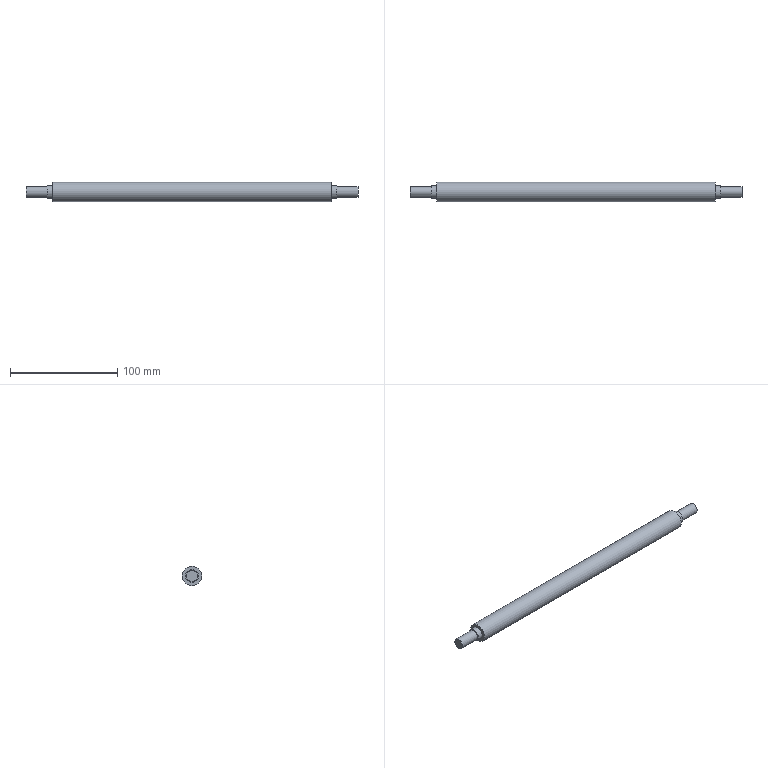Part | NX | 1 solid | 11 faces | box 310 x 18 x 18 mm | volume 70435 mm3 | plane 6 | cylinder 5 | commonest cylinder face diameters 10 x2 12 x2 18 x1
STEP:
#1=CARTESIAN_POINT('',(135.,0.,-6.));
#2=VERTEX_POINT('',#1);
#3=CARTESIAN_POINT('',(135.,0.,0.));
#4=DIRECTION('',(1.,0.,0.));
#5=DIRECTION('',(0.,0.,-1.));
#6=AXIS2_PLACEMENT_3D('',#3,#4,#5);
#7=CIRCLE('',#6,6.);
#8=EDGE_CURVE('',#2,#2,#7,.T.);
#9=ORIENTED_EDGE('',*,*,#8,.T.);
#10=EDGE_LOOP('',(#9));
#11=FACE_BOUND('',#10,.T.);
#12=CARTESIAN_POINT('',(135.,0.,-5.));
#13=VERTEX_POINT('',#12);
#14=CARTESIAN_POINT('',(135.,0.,0.));
#15=DIRECTION('',(1.,0.,0.));
#16=DIRECTION('',(0.,0.,-1.));
#17=AXIS2_PLACEMENT_3D('',#14,#15,#16);
#18=CIRCLE('',#17,5.);
#19=EDGE_CURVE('',#13,#13,#18,.T.);
#20=ORIENTED_EDGE('',*,*,#19,.F.);
#21=EDGE_LOOP('',(#20));
#22=FACE_BOUND('',#21,.T.);
#23=CARTESIAN_POINT('',(135.,0.,0.));
#24=DIRECTION('',(1.,0.,0.));
#25=DIRECTION('',(0.,0.,-1.));
#26=AXIS2_PLACEMENT_3D('',#23,#24,#25);
#27=PLANE('',#26);
#28=ADVANCED_FACE('',(#11,#22),#27,.T.);
#29=CARTESIAN_POINT('',(130.,0.,-9.));
#30=VERTEX_POINT('',#29);
#31=CARTESIAN_POINT('',(130.,0.,0.));
#32=DIRECTION('',(1.,0.,0.));
#33=DIRECTION('',(0.,0.,-1.));
#34=AXIS2_PLACEMENT_3D('',#31,#32,#33);
#35=CIRCLE('',#34,9.);
#36=EDGE_CURVE('',#30,#30,#35,.T.);
#37=ORIENTED_EDGE('',*,*,#36,.T.);
#38=EDGE_LOOP('',(#37));
#39=FACE_BOUND('',#38,.T.);
#40=CARTESIAN_POINT('',(130.,0.,-6.));
#41=VERTEX_POINT('',#40);
#42=CARTESIAN_POINT('',(130.,0.,0.));
#43=DIRECTION('',(1.,0.,0.));
#44=DIRECTION('',(0.,0.,-1.));
#45=AXIS2_PLACEMENT_3D('',#42,#43,#44);
#46=CIRCLE('',#45,6.);
#47=EDGE_CURVE('',#41,#41,#46,.T.);
#48=ORIENTED_EDGE('',*,*,#47,.F.);
#49=EDGE_LOOP('',(#48));
#50=FACE_BOUND('',#49,.T.);
#51=CARTESIAN_POINT('',(130.,0.,0.));
#52=DIRECTION('',(1.,0.,0.));
#53=DIRECTION('',(0.,0.,-1.));
#54=AXIS2_PLACEMENT_3D('',#51,#52,#53);
#55=PLANE('',#54);
#56=ADVANCED_FACE('',(#39,#50),#55,.T.);
#57=ORIENTED_EDGE('',*,*,#36,.F.);
#58=EDGE_LOOP('',(#57));
#59=FACE_BOUND('',#58,.T.);
#60=CARTESIAN_POINT('',(-130.,0.,-9.));
#61=VERTEX_POINT('',#60);
#62=CARTESIAN_POINT('',(-130.,0.,0.));
#63=DIRECTION('',(1.,0.,0.));
#64=DIRECTION('',(0.,0.,-1.));
#65=AXIS2_PLACEMENT_3D('',#62,#63,#64);
#66=CIRCLE('',#65,9.);
#67=EDGE_CURVE('',#61,#61,#66,.T.);
#68=ORIENTED_EDGE('',*,*,#67,.T.);
#69=EDGE_LOOP('',(#68));
#70=FACE_BOUND('',#69,.T.);
#71=CARTESIAN_POINT('',(130.,0.,0.));
#72=DIRECTION('',(-1.,0.,0.));
#73=DIRECTION('',(0.,0.,1.));
#74=AXIS2_PLACEMENT_3D('',#71,#72,#73);
#75=CYLINDRICAL_SURFACE('',#74,9.);
#76=ADVANCED_FACE('',(#59,#70),#75,.T.);
#77=CARTESIAN_POINT('',(-130.,0.,-6.));
#78=VERTEX_POINT('',#77);
#79=CARTESIAN_POINT('',(-130.,0.,0.));
#80=DIRECTION('',(1.,0.,0.));
#81=DIRECTION('',(0.,0.,-1.));
#82=AXIS2_PLACEMENT_3D('',#79,#80,#81);
#83=CIRCLE('',#82,6.);
#84=EDGE_CURVE('',#78,#78,#83,.T.);
#85=ORIENTED_EDGE('',*,*,#84,.T.);
#86=EDGE_LOOP('',(#85));
#87=FACE_BOUND('',#86,.T.);
#88=ORIENTED_EDGE('',*,*,#67,.F.);
#89=EDGE_LOOP('',(#88));
#90=FACE_BOUND('',#89,.T.);
#91=CARTESIAN_POINT('',(-130.,0.,0.));
#92=DIRECTION('',(1.,0.,0.));
#93=DIRECTION('',(0.,0.,-1.));
#94=AXIS2_PLACEMENT_3D('',#91,#92,#93);
#95=PLANE('',#94);
#96=ADVANCED_FACE('',(#87,#90),#95,.F.);
#97=ORIENTED_EDGE('',*,*,#8,.F.);
#98=EDGE_LOOP('',(#97));
#99=FACE_BOUND('',#98,.T.);
#100=ORIENTED_EDGE('',*,*,#47,.T.);
#101=EDGE_LOOP('',(#100));
#102=FACE_BOUND('',#101,.T.);
#103=CARTESIAN_POINT('',(135.,0.,0.));
#104=DIRECTION('',(-1.,0.,0.));
#105=DIRECTION('',(0.,0.,1.));
#106=AXIS2_PLACEMENT_3D('',#103,#104,#105);
#107=CYLINDRICAL_SURFACE('',#106,6.);
#108=ADVANCED_FACE('',(#99,#102),#107,.T.);
#109=CARTESIAN_POINT('',(155.,0.,-5.));
#110=VERTEX_POINT('',#109);
#111=CARTESIAN_POINT('',(155.,0.,0.));
#112=DIRECTION('',(1.,0.,0.));
#113=DIRECTION('',(0.,0.,-1.));
#114=AXIS2_PLACEMENT_3D('',#111,#112,#113);
#115=CIRCLE('',#114,5.);
#116=EDGE_CURVE('',#110,#110,#115,.T.);
#117=ORIENTED_EDGE('',*,*,#116,.F.);
#118=EDGE_LOOP('',(#117));
#119=FACE_BOUND('',#118,.T.);
#120=ORIENTED_EDGE('',*,*,#19,.T.);
#121=EDGE_LOOP('',(#120));
#122=FACE_BOUND('',#121,.T.);
#123=CARTESIAN_POINT('',(155.,0.,0.));
#124=DIRECTION('',(-1.,0.,0.));
#125=DIRECTION('',(0.,0.,1.));
#126=AXIS2_PLACEMENT_3D('',#123,#124,#125);
#127=CYLINDRICAL_SURFACE('',#126,5.);
#128=ADVANCED_FACE('',(#119,#122),#127,.T.);
#129=ORIENTED_EDGE('',*,*,#116,.T.);
#130=EDGE_LOOP('',(#129));
#131=FACE_BOUND('',#130,.T.);
#132=CARTESIAN_POINT('',(155.,0.,0.));
#133=DIRECTION('',(1.,0.,0.));
#134=DIRECTION('',(0.,0.,-1.));
#135=AXIS2_PLACEMENT_3D('',#132,#133,#134);
#136=PLANE('',#135);
#137=ADVANCED_FACE('',(#131),#136,.T.);
#138=CARTESIAN_POINT('',(-135.,0.,-6.));
#139=VERTEX_POINT('',#138);
#140=CARTESIAN_POINT('',(-135.,0.,0.));
#141=DIRECTION('',(1.,0.,0.));
#142=DIRECTION('',(0.,0.,-1.));
#143=AXIS2_PLACEMENT_3D('',#140,#141,#142);
#144=CIRCLE('',#143,6.);
#145=EDGE_CURVE('',#139,#139,#144,.T.);
#146=ORIENTED_EDGE('',*,*,#145,.T.);
#147=EDGE_LOOP('',(#146));
#148=FACE_BOUND('',#147,.T.);
#149=ORIENTED_EDGE('',*,*,#84,.F.);
#150=EDGE_LOOP('',(#149));
#151=FACE_BOUND('',#150,.T.);
#152=CARTESIAN_POINT('',(-135.,0.,0.));
#153=DIRECTION('',(1.,0.,0.));
#154=DIRECTION('',(0.,0.,-1.));
#155=AXIS2_PLACEMENT_3D('',#152,#153,#154);
#156=CYLINDRICAL_SURFACE('',#155,6.);
#157=ADVANCED_FACE('',(#148,#151),#156,.T.);
#158=CARTESIAN_POINT('',(-135.,0.,5.));
#159=VERTEX_POINT('',#158);
#160=CARTESIAN_POINT('',(-135.,0.,0.));
#161=DIRECTION('',(-1.,0.,0.));
#162=DIRECTION('',(0.,0.,1.));
#163=AXIS2_PLACEMENT_3D('',#160,#161,#162);
#164=CIRCLE('',#163,5.);
#165=EDGE_CURVE('',#159,#159,#164,.T.);
#166=ORIENTED_EDGE('',*,*,#165,.F.);
#167=EDGE_LOOP('',(#166));
#168=FACE_BOUND('',#167,.T.);
#169=ORIENTED_EDGE('',*,*,#145,.F.);
#170=EDGE_LOOP('',(#169));
#171=FACE_BOUND('',#170,.T.);
#172=CARTESIAN_POINT('',(-135.,0.,0.));
#173=DIRECTION('',(-1.,0.,0.));
#174=DIRECTION('',(0.,0.,-1.));
#175=AXIS2_PLACEMENT_3D('',#172,#173,#174);
#176=PLANE('',#175);
#177=ADVANCED_FACE('',(#168,#171),#176,.T.);
#178=CARTESIAN_POINT('',(-155.,0.,-5.));
#179=VERTEX_POINT('',#178);
#180=CARTESIAN_POINT('',(-155.,0.,0.));
#181=DIRECTION('',(1.,0.,0.));
#182=DIRECTION('',(0.,0.,-1.));
#183=AXIS2_PLACEMENT_3D('',#180,#181,#182);
#184=CIRCLE('',#183,5.);
#185=EDGE_CURVE('',#179,#179,#184,.T.);
#186=ORIENTED_EDGE('',*,*,#185,.T.);
#187=EDGE_LOOP('',(#186));
#188=FACE_BOUND('',#187,.T.);
#189=ORIENTED_EDGE('',*,*,#165,.T.);
#190=EDGE_LOOP('',(#189));
#191=FACE_BOUND('',#190,.T.);
#192=CARTESIAN_POINT('',(-155.,0.,0.));
#193=DIRECTION('',(1.,0.,0.));
#194=DIRECTION('',(0.,0.,-1.));
#195=AXIS2_PLACEMENT_3D('',#192,#193,#194);
#196=CYLINDRICAL_SURFACE('',#195,5.);
#197=ADVANCED_FACE('',(#188,#191),#196,.T.);
#198=ORIENTED_EDGE('',*,*,#185,.F.);
#199=EDGE_LOOP('',(#198));
#200=FACE_BOUND('',#199,.T.);
#201=CARTESIAN_POINT('',(-155.,0.,0.));
#202=DIRECTION('',(-1.,0.,0.));
#203=DIRECTION('',(0.,0.,-1.));
#204=AXIS2_PLACEMENT_3D('',#201,#202,#203);
#205=PLANE('',#204);
#206=ADVANCED_FACE('',(#200),#205,.T.);
#207=CLOSED_SHELL('',(#28,#56,#76,#96,#108,#128,#137,#157,#177,#197,#206));
#208=MANIFOLD_SOLID_BREP('',#207);
#209=(LENGTH_UNIT()NAMED_UNIT(*)SI_UNIT(.MILLI.,.METRE.));
#210=UNCERTAINTY_MEASURE_WITH_UNIT(LENGTH_MEASURE(0.00001),#209,'','');
#211=(NAMED_UNIT(*)PLANE_ANGLE_UNIT()SI_UNIT($,.RADIAN.));
#212=(NAMED_UNIT(*)SI_UNIT($,.STERADIAN.)SOLID_ANGLE_UNIT());
#213=(GEOMETRIC_REPRESENTATION_CONTEXT(3)GLOBAL_UNCERTAINTY_ASSIGNED_CONTEXT((#210))GLOBAL_UNIT_ASSIGNED_CONTEXT((#209,#211,#212))REPRESENTATION_CONTEXT('',''));
#214=ADVANCED_BREP_SHAPE_REPRESENTATION('',(#208),#213);